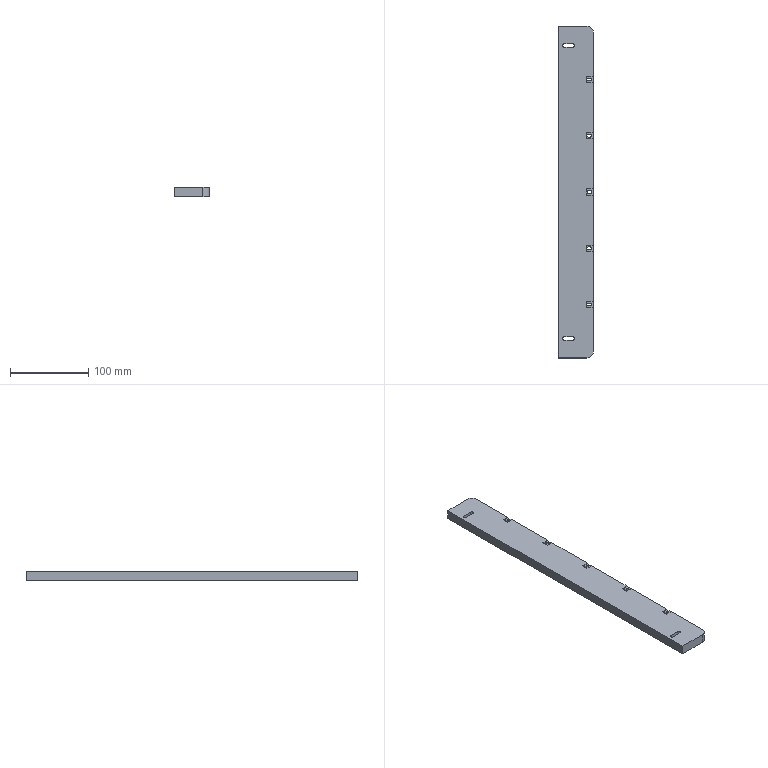Part | SolidWorks | features ICE 5, Extrusion 1, Fillet 1, LPattern 1 | 1 solid | 105 faces | box 44 x 425 x 12 mm | volume 219705 mm3 | plane 61 | cylinder 44 | commonest cylinder face diameters 3.2 x15 6 x15 4 x6 8 x6 16 x2